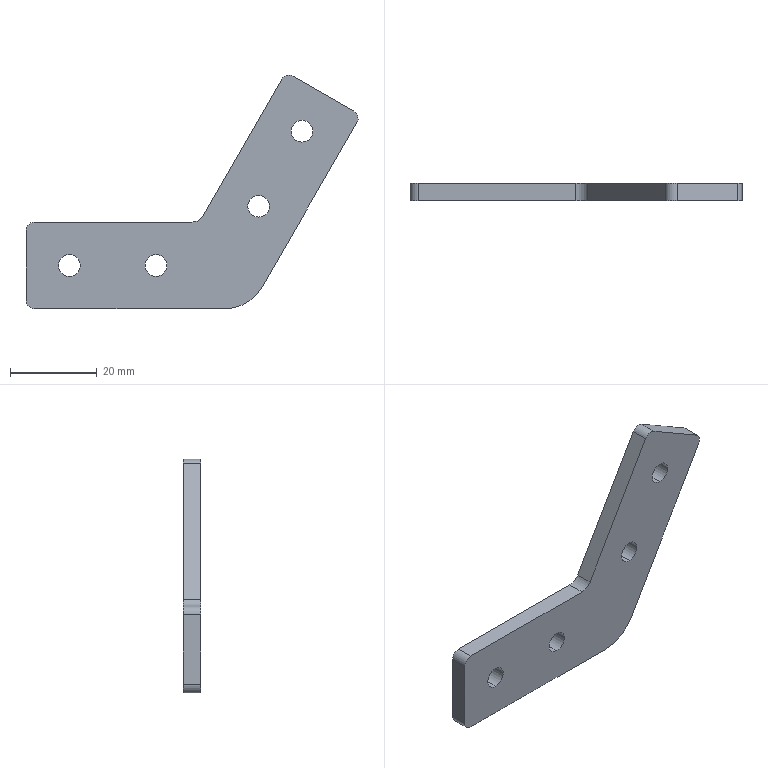Part | STEP file | 120-degree side frame | 1 solid | 22 faces | box 76.588 x 4 x 53.909 mm | volume 6976 mm3 | cylinder 14 | plane 8 | commonest cylinder face diameters 5 x8 4 x4 6 x1 20 x1